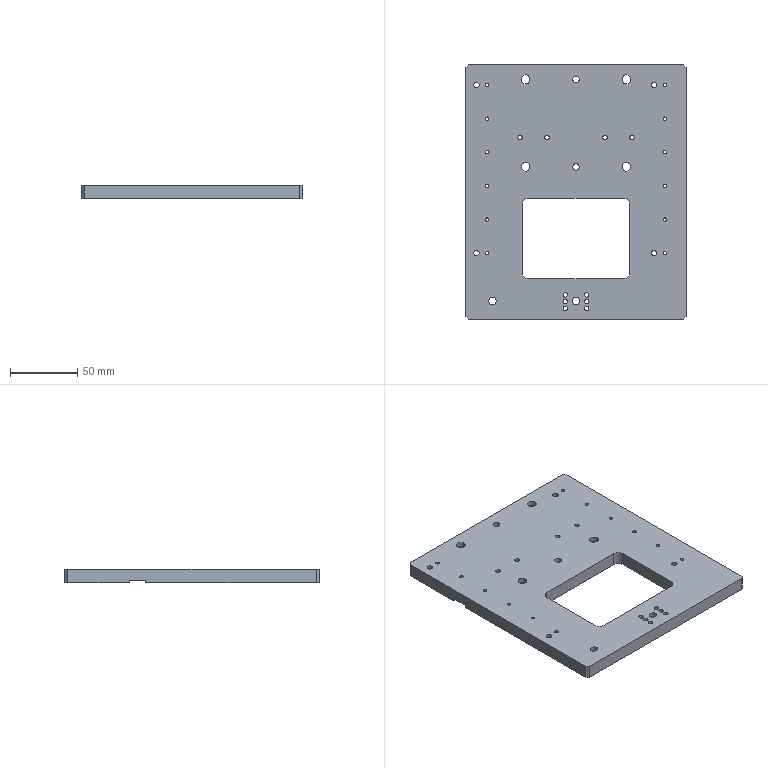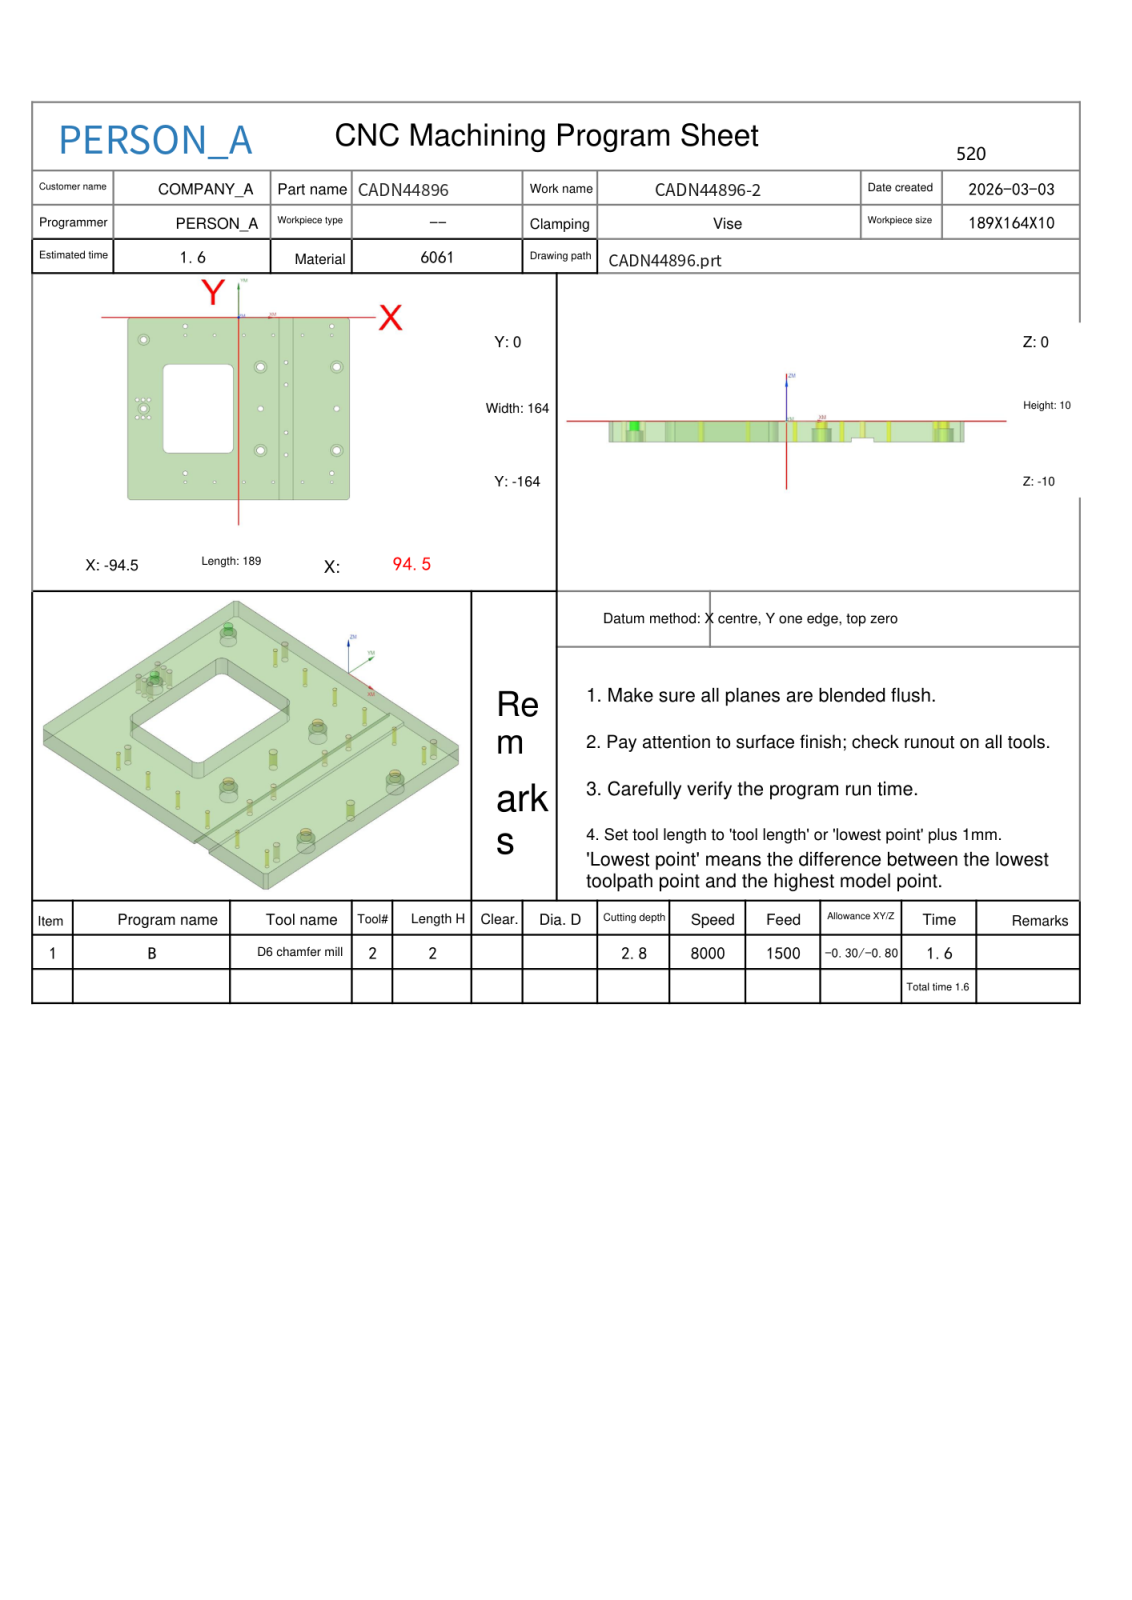NC program | NX | posted by the shop | part box 164 x 189 x 10 mm
Whole program:
%
O0001
(Machine time: 1.67 MIN)
(===Total Tool:1===)
(T2=D6 chamfer mill   D=6.   R=0.   D-  H02 Z=-2.8  )
G80 G90 G17 G49 G40
G91 G28 Z0
M01
N1 T02 M06
(D6 chamfer mill  D=6. R=0. H=02 ce=-0.30 di=0.00)
G00 G90 G54 X-44.338 Y-7.418 M03 S7000
G43 H02 Z50.
M08
Z2.5
G01 X-44.434 Y-7.251 Z2.43 F1500.
X-44.584 Y-7.074 Z2.345
X-44.762 Y-6.926 Z2.261
X-44.964 Y-6.812 Z2.177
X-45.183 Y-6.736 Z2.092
X-45.412 Y-6.7 Z2.008
X-45.588 Z1.944
X-45.817 Y-6.736 Z1.859
X-46.036 Y-6.812 Z1.775
X-46.238 Y-6.926 Z1.691
X-46.416 Y-7.074 Z1.606
X-46.566 Y-7.251 Z1.522
X-46.682 Y-7.451 Z1.438
X-46.76 Y-7.669 Z1.353
X-46.799 Y-7.898 Z1.269
X-46.797 Y-8.13 Z1.185
X-46.753 Y-8.357 Z1.1
X-46.67 Y-8.573 Z1.016
X-46.582 Y-8.727 Z.952
X-46.436 Y-8.907 Z.867
X-46.26 Y-9.058 Z.783
X-46.061 Y-9.176 Z.699
X-45.844 Y-9.257 Z.614
X-45.616 Y-9.298 Z.53
X-45.384 Z.446
X-45.156 Y-9.257 Z.361
X-44.939 Y-9.176 Z.277
X-44.74 Y-9.058 Z.193
X-44.564 Y-8.907 Z.108
X-44.418 Y-8.727 Z.024
X-44.33 Y-8.573 Z-.04
X-44.247 Y-8.357 Z-.125
X-44.203 Y-8.13 Z-.209
X-44.201 Y-7.898 Z-.293
X-44.24 Y-7.669 Z-.378
X-44.318 Y-7.451 Z-.462
X-44.434 Y-7.251 Z-.546
X-44.584 Y-7.074 Z-.631
X-44.762 Y-6.926 Z-.715
X-44.964 Y-6.812 Z-.799
X-45.183 Y-6.736 Z-.884
X-45.412 Y-6.7 Z-.968
X-45.5 Z-1.
G03 X-46.8 Y-8. I0.0 J-1.3
X-45.5 Y-9.3 I1.3 J0.0
X-44.2 Y-8. I0.0 J1.3
X-45.5 Y-6.7 I-1.3 J0.0
X-45.988 Y-6.795 I0.0 J-1.3
G01 Z1.5
G00 Z50.
X-83.051 Y-20.049
Z2.5
G01 X-83.025 Y-20.335 Z2.396
X-82.951 Y-20.639 Z2.281
X-82.831 Y-20.929 Z2.167
X-82.72 Y-21.121 Z2.087
X-82.529 Y-21.37 Z1.973
X-82.303 Y-21.587 Z1.859
X-82.046 Y-21.766 Z1.744
X-81.765 Y-21.905 Z1.63
X-81.466 Y-21.999 Z1.516
X-81.157 Y-22.047 Z1.402
X-80.843 Z1.288
X-80.534 Y-21.999 Z1.174
X-80.235 Y-21.905 Z1.06
X-79.954 Y-21.766 Z.946
X-79.697 Y-21.587 Z.832
X-79.471 Y-21.37 Z.718
X-79.28 Y-21.121 Z.604
X-79.169 Y-20.929 Z.523
X-79.049 Y-20.639 Z.409
X-78.975 Y-20.335 Z.295
X-78.947 Y-20.023 Z.181
X-78.968 Y-19.71 Z.067
X-79.035 Y-19.404 Z-.047
X-79.149 Y-19.112 Z-.161
X-79.306 Y-18.841 Z-.275
X-79.502 Y-18.596 Z-.389
X-79.733 Y-18.385 Z-.503
X-79.993 Y-18.211 Z-.617
X-80.277 Y-18.078 Z-.732
X-80.578 Y-17.991 Z-.846
X-80.889 Y-17.95 Z-.96
X-81. Z-1.
G03 X-83.05 Y-20. I0.0 J-2.05
X-81. Y-22.05 I2.05 J0.0
X-78.95 Y-20. I0.0 J2.05
X-81. Y-17.95 I-2.05 J0.0
X-81.495 Y-18.011 I0.0 J-2.05
G01 Z1.5
G00 Z50.
X-83.051 Y-82.049
Z2.5
G01 X-83.025 Y-82.335 Z2.396
X-82.951 Y-82.639 Z2.281
X-82.831 Y-82.929 Z2.167
X-82.72 Y-83.121 Z2.087
X-82.529 Y-83.37 Z1.973
X-82.303 Y-83.587 Z1.859
X-82.046 Y-83.766 Z1.744
X-81.765 Y-83.905 Z1.63
X-81.466 Y-83.999 Z1.516
X-81.157 Y-84.047 Z1.402
X-80.843 Z1.288
X-80.534 Y-83.999 Z1.174
X-80.235 Y-83.905 Z1.06
X-79.954 Y-83.766 Z.946
X-79.697 Y-83.587 Z.832
X-79.471 Y-83.37 Z.718
X-79.28 Y-83.121 Z.604
X-79.169 Y-82.929 Z.523
X-79.049 Y-82.639 Z.409
X-78.975 Y-82.335 Z.295
X-78.947 Y-82.023 Z.181
X-78.968 Y-81.71 Z.067
X-79.035 Y-81.404 Z-.047
X-79.149 Y-81.112 Z-.161
X-79.306 Y-80.841 Z-.275
X-79.502 Y-80.596 Z-.389
X-79.733 Y-80.385 Z-.503
X-79.993 Y-80.211 Z-.617
X-80.277 Y-80.078 Z-.732
X-80.578 Y-79.991 Z-.846
X-80.889 Y-79.95 Z-.96
X-81. Z-1.
G03 X-83.05 Y-82. I0.0 J-2.05
X-81. Y-84.05 I2.05 J0.0
X-78.95 Y-82. I0.0 J2.05
X-81. Y-79.95 I-2.05 J0.0
X-81.495 Y-80.011 I0.0 J-2.05
G01 Z1.5
G00 Z50.
X-44.338 Y-139.418
Z2.5
G01 X-44.434 Y-139.251 Z2.43
X-44.584 Y-139.074 Z2.345
X-44.762 Y-138.926 Z2.261
X-44.964 Y-138.812 Z2.177
X-45.183 Y-138.736 Z2.092
X-45.412 Y-138.7 Z2.008
X-45.588 Z1.944
X-45.817 Y-138.736 Z1.859
X-46.036 Y-138.812 Z1.775
X-46.238 Y-138.926 Z1.691
X-46.416 Y-139.074 Z1.606
X-46.566 Y-139.251 Z1.522
X-46.682 Y-139.451 Z1.438
X-46.76 Y-139.669 Z1.353
X-46.799 Y-139.898 Z1.269
X-46.797 Y-140.13 Z1.185
X-46.753 Y-140.357 Z1.1
X-46.67 Y-140.573 Z1.016
X-46.582 Y-140.727 Z.952
X-46.436 Y-140.907 Z.867
X-46.26 Y-141.058 Z.783
X-46.061 Y-141.176 Z.699
X-45.844 Y-141.257 Z.614
X-45.616 Y-141.298 Z.53
X-45.384 Z.446
X-45.156 Y-141.257 Z.361
X-44.939 Y-141.176 Z.277
X-44.74 Y-141.058 Z.193
X-44.564 Y-140.907 Z.108
X-44.418 Y-140.727 Z.024
X-44.33 Y-140.573 Z-.04
X-44.247 Y-140.357 Z-.125
X-44.203 Y-140.13 Z-.209
X-44.201 Y-139.898 Z-.293
X-44.24 Y-139.669 Z-.378
X-44.318 Y-139.451 Z-.462
X-44.434 Y-139.251 Z-.546
X-44.584 Y-139.074 Z-.631
X-44.762 Y-138.926 Z-.715
X-44.964 Y-138.812 Z-.799
X-45.183 Y-138.736 Z-.884
X-45.412 Y-138.7 Z-.968
X-45.5 Z-1.
G03 X-46.8 Y-140. I0.0 J-1.3
X-45.5 Y-141.3 I1.3 J0.0
X-44.2 Y-140. I0.0 J1.3
X-45.5 Y-138.7 I-1.3 J0.0
X-45.988 Y-138.795 I0.0 J-1.3
G01 Z1.5
G00 Z50.
X-49.884 Y-42.7
Z2.5
G01 X-59.5 Z-1.
G03 X-63.8 Y-47. I0.0 J-4.3
G01 Y-117.
G03 X-59.5 Y-121.3 I4.3 J0.0
G01 X-9.5
G03 X-5.2 Y-117. I0.0 J4.3
G01 Y-47.
G03 X-9.5 Y-42.7 I-4.3 J0.0
G01 X-59.5
G03 X-59.999 Y-42.729 I0.0 J-4.3
G01 Z1.5
G00 Z50.
X-83.546 Y-164.7
Z2.5
G01 X-92.453 Z-.742
X-92.66 Y-164.662 Z-.819
X-92.855 Y-164.581 Z-.895
X-93.028 Y-164.462 Z-.972
X-93.083 Y-164.407 Z-1.
X-94.907 Y-162.583
G02 X-95.2 Y-161.876 I.707 J.707
G01 Y-2.124
G02 X-94.907 Y-1.417 I1. J0.0
G01 X-93.083 Y.407
G02 X-92.376 Y.7 I.707 J-.707
G01 X92.376
G02 X93.083 Y.407 I0.0 J-1.
G01 X94.907 Y-1.417
G02 X95.2 Y-2.124 I-.707 J-.707
G01 Y-161.876
G02 X94.907 Y-162.583 I-1. J0.0
G01 X93.083 Y-164.407
G02 X92.376 Y-164.7 I-.707 J.707
G01 X-92.376
G02 X-93.083 Y-164.407 I0.0 J1.
G01 X-93.436 Y-164.054
Z1.5
G00 Z50.
X17.33 Y-46.707
Z2.5
G01 X17.53 Y-46.825 Z2.416
X17.849 Y-46.96 Z2.29
X18.183 Y-47.051 Z2.163
X18.527 Y-47.097 Z2.037
X18.873 Z1.911
X19.217 Y-47.051 Z1.785
X19.551 Y-46.96 Z1.659
X19.87 Y-46.825 Z1.533
X20.169 Y-46.649 Z1.407
X20.441 Y-46.435 Z1.281
X20.683 Y-46.187 Z1.154
X20.889 Y-45.908 Z1.028
X21.014 Y-45.692 Z.937
X21.152 Y-45.374 Z.811
X21.246 Y-45.04 Z.685
X21.296 Y-44.697 Z.559
X21.299 Y-44.351 Z.433
X21.256 Y-44.007 Z.307
X21.168 Y-43.672 Z.181
X21.036 Y-43.351 Z.054
X20.863 Y-43.051 Z-.072
X20.651 Y-42.777 Z-.198
X20.405 Y-42.533 Z-.324
X20.128 Y-42.324 Z-.45
X19.827 Y-42.154 Z-.576
X19.505 Y-42.025 Z-.702
X19.169 Y-41.94 Z-.828
X18.825 Y-41.9 Z-.955
X18.7 Z-1.
G03 X16.1 Y-44.5 I0.0 J-2.6
X18.7 Y-47.1 I2.6 J0.0
X21.3 Y-44.5 I0.0 J2.6
X18.7 Y-41.9 I-2.6 J0.0
X18.203 Y-41.948 I0.0 J-2.6
G01 Z1.5
G00 Z50.
X20.159 Y-83.055
Z2.5
G01 X20.188 Y-83.018 Z2.483
X20.325 Y-82.78 Z2.383
X20.425 Y-82.525 Z2.283
X20.485 Y-82.257 Z2.183
X20.503 Y-81.983 Z2.084
X20.48 Y-81.71 Z1.984
X20.415 Y-81.444 Z1.884
X20.311 Y-81.19 Z1.784
X20.207 Y-81.01 Z1.708
X20.039 Y-80.793 Z1.609
X19.841 Y-80.604 Z1.509
X19.616 Y-80.447 Z1.409
X19.37 Y-80.326 Z1.309
X19.108 Y-80.244 Z1.209
X18.837 Y-80.202 Z1.11
X18.563 Z1.01
X18.292 Y-80.244 Z.91
X18.03 Y-80.326 Z.81
X17.784 Y-80.447 Z.71
X17.559 Y-80.604 Z.611
X17.361 Y-80.793 Z.511
X17.193 Y-81.01 Z.411
X17.089 Y-81.19 Z.335
X16.985 Y-81.444 Z.235
X16.92 Y-81.71 Z.136
X16.897 Y-81.983 Z.036
X16.915 Y-82.257 Z-.064
X16.975 Y-82.525 Z-.164
X17.075 Y-82.78 Z-.264
X17.212 Y-83.018 Z-.363
X17.383 Y-83.232 Z-.463
X17.585 Y-83.417 Z-.563
X17.813 Y-83.57 Z-.663
X18.061 Y-83.686 Z-.763
X18.324 Y-83.763 Z-.862
X18.596 Y-83.8 Z-.962
X18.7 Z-1.
G03 X20.5 Y-82. I0.0 J1.8
X18.7 Y-80.2 I-1.8 J0.0
X16.9 Y-82. I0.0 J-1.8
X18.7 Y-83.8 I1.8 J0.0
X19.194 Y-83.731 I0.0 J1.8
G01 Z1.5
G00 Z50.
X17.33 Y-121.707
Z2.5
G01 X17.53 Y-121.825 Z2.416
X17.849 Y-121.96 Z2.29
X18.183 Y-122.051 Z2.163
X18.527 Y-122.097 Z2.037
X18.873 Z1.911
X19.217 Y-122.051 Z1.785
X19.551 Y-121.96 Z1.659
X19.87 Y-121.825 Z1.533
X20.169 Y-121.649 Z1.407
X20.441 Y-121.435 Z1.281
X20.683 Y-121.187 Z1.154
X20.889 Y-120.908 Z1.028
X21.014 Y-120.692 Z.937
X21.152 Y-120.374 Z.811
X21.246 Y-120.04 Z.685
X21.296 Y-119.697 Z.559
X21.299 Y-119.351 Z.433
X21.256 Y-119.007 Z.307
X21.168 Y-118.672 Z.181
X21.036 Y-118.351 Z.054
X20.863 Y-118.051 Z-.072
X20.651 Y-117.777 Z-.198
X20.405 Y-117.533 Z-.324
X20.128 Y-117.324 Z-.45
X19.827 Y-117.154 Z-.576
X19.505 Y-117.025 Z-.702
X19.169 Y-116.94 Z-.828
X18.825 Y-116.9 Z-.955
X18.7 Z-1.
G03 X16.1 Y-119.5 I0.0 J-2.6
X18.7 Y-122.1 I2.6 J0.0
X21.3 Y-119.5 I0.0 J2.6
X18.7 Y-116.9 I-2.6 J0.0
X18.203 Y-116.948 I0.0 J-2.6
G01 Z1.5
G00 Z50.
X80.662 Y-139.418
Z2.5
G01 X80.566 Y-139.251 Z2.43
X80.416 Y-139.074 Z2.345
X80.238 Y-138.926 Z2.261
X80.036 Y-138.812 Z2.177
X79.817 Y-138.736 Z2.092
X79.588 Y-138.7 Z2.008
X79.412 Z1.944
X79.183 Y-138.736 Z1.859
X78.964 Y-138.812 Z1.775
X78.762 Y-138.926 Z1.691
X78.584 Y-139.074 Z1.606
X78.434 Y-139.251 Z1.522
X78.318 Y-139.451 Z1.438
X78.24 Y-139.669 Z1.353
X78.201 Y-139.898 Z1.269
X78.203 Y-140.13 Z1.185
X78.247 Y-140.357 Z1.1
X78.33 Y-140.573 Z1.016
X78.418 Y-140.727 Z.952
X78.564 Y-140.907 Z.867
X78.74 Y-141.058 Z.783
X78.939 Y-141.176 Z.699
X79.156 Y-141.257 Z.614
X79.384 Y-141.298 Z.53
X79.616 Z.446
X79.844 Y-141.257 Z.361
X80.061 Y-141.176 Z.277
X80.26 Y-141.058 Z.193
X80.436 Y-140.907 Z.108
X80.582 Y-140.727 Z.024
X80.67 Y-140.573 Z-.04
X80.753 Y-140.357 Z-.125
X80.797 Y-140.13 Z-.209
X80.799 Y-139.898 Z-.293
X80.76 Y-139.669 Z-.378
X80.682 Y-139.451 Z-.462
X80.566 Y-139.251 Z-.546
X80.416 Y-139.074 Z-.631
X80.238 Y-138.926 Z-.715
X80.036 Y-138.812 Z-.799
X79.817 Y-138.736 Z-.884
X79.588 Y-138.7 Z-.968
X79.5 Z-1.
G03 X78.2 Y-140. I0.0 J-1.3
X79.5 Y-141.3 I1.3 J0.0
X80.8 Y-140. I0.0 J1.3
X79.5 Y-138.7 I-1.3 J0.0
X79.012 Y-138.795 I0.0 J-1.3
G01 Z1.5
G00 Z50.
X82.33 Y-121.707
Z2.5
G01 X82.53 Y-121.825 Z2.416
X82.849 Y-121.96 Z2.29
X83.183 Y-122.051 Z2.163
X83.527 Y-122.097 Z2.037
X83.873 Z1.911
X84.217 Y-122.051 Z1.785
X84.551 Y-121.96 Z1.659
X84.87 Y-121.825 Z1.533
X85.169 Y-121.649 Z1.407
X85.441 Y-121.435 Z1.281
X85.683 Y-121.187 Z1.154
X85.889 Y-120.908 Z1.028
X86.014 Y-120.692 Z.937
X86.152 Y-120.374 Z.811
X86.246 Y-120.04 Z.685
X86.296 Y-119.697 Z.559
X86.299 Y-119.351 Z.433
X86.256 Y-119.007 Z.307
X86.168 Y-118.672 Z.181
X86.036 Y-118.351 Z.054
X85.863 Y-118.051 Z-.072
X85.651 Y-117.777 Z-.198
X85.405 Y-117.533 Z-.324
X85.128 Y-117.324 Z-.45
X84.827 Y-117.154 Z-.576
X84.505 Y-117.025 Z-.702
X84.169 Y-116.94 Z-.828
X83.825 Y-116.9 Z-.955
X83.7 Z-1.
G03 X81.1 Y-119.5 I0.0 J-2.6
X83.7 Y-122.1 I2.6 J0.0
X86.3 Y-119.5 I0.0 J2.6
X83.7 Y-116.9 I-2.6 J0.0
X83.203 Y-116.948 I0.0 J-2.6
G01 Z1.5
G00 Z50.
X85.159 Y-83.055
Z2.5
G01 X85.188 Y-83.018 Z2.483
X85.325 Y-82.78 Z2.383
X85.425 Y-82.525 Z2.283
X85.485 Y-82.257 Z2.183
X85.503 Y-81.983 Z2.084
X85.48 Y-81.71 Z1.984
X85.415 Y-81.444 Z1.884
X85.311 Y-81.19 Z1.784
X85.207 Y-81.01 Z1.708
X85.039 Y-80.793 Z1.609
X84.841 Y-80.604 Z1.509
X84.616 Y-80.447 Z1.409
X84.37 Y-80.326 Z1.309
X84.108 Y-80.244 Z1.209
X83.837 Y-80.202 Z1.11
X83.563 Z1.01
X83.292 Y-80.244 Z.91
X83.03 Y-80.326 Z.81
X82.784 Y-80.447 Z.71
X82.559 Y-80.604 Z.611
X82.361 Y-80.793 Z.511
X82.193 Y-81.01 Z.411
X82.089 Y-81.19 Z.335
X81.985 Y-81.444 Z.235
X81.92 Y-81.71 Z.136
X81.897 Y-81.983 Z.036
X81.915 Y-82.257 Z-.064
X81.975 Y-82.525 Z-.164
X82.075 Y-82.78 Z-.264
X82.212 Y-83.018 Z-.363
X82.383 Y-83.232 Z-.463
X82.585 Y-83.417 Z-.563
X82.813 Y-83.57 Z-.663
X83.061 Y-83.686 Z-.763
X83.324 Y-83.763 Z-.862
X83.596 Y-83.8 Z-.962
X83.7 Z-1.
G03 X85.5 Y-82. I0.0 J1.8
X83.7 Y-80.2 I-1.8 J0.0
X81.9 Y-82. I0.0 J-1.8
X83.7 Y-83.8 I1.8 J0.0
X84.194 Y-83.731 I0.0 J1.8
G01 Z1.5
G00 Z50.
X82.33 Y-46.707
Z2.5
G01 X82.53 Y-46.825 Z2.416
X82.849 Y-46.96 Z2.29
X83.183 Y-47.051 Z2.163
X83.527 Y-47.097 Z2.037
X83.873 Z1.911
X84.217 Y-47.051 Z1.785
X84.551 Y-46.96 Z1.659
X84.87 Y-46.825 Z1.533
X85.169 Y-46.649 Z1.407
X85.441 Y-46.435 Z1.281
X85.683 Y-46.187 Z1.154
X85.889 Y-45.908 Z1.028
X86.014 Y-45.692 Z.937
X86.152 Y-45.374 Z.811
X86.246 Y-45.04 Z.685
X86.296 Y-44.697 Z.559
X86.299 Y-44.351 Z.433
X86.256 Y-44.007 Z.307
X86.168 Y-43.672 Z.181
X86.036 Y-43.351 Z.054
X85.863 Y-43.051 Z-.072
X85.651 Y-42.777 Z-.198
X85.405 Y-42.533 Z-.324
X85.128 Y-42.324 Z-.45
X84.827 Y-42.154 Z-.576
X84.505 Y-42.025 Z-.702
X84.169 Y-41.94 Z-.828
X83.825 Y-41.9 Z-.955
X83.7 Z-1.
G03 X81.1 Y-44.5 I0.0 J-2.6
X83.7 Y-47.1 I2.6 J0.0
X86.3 Y-44.5 I0.0 J2.6
X83.7 Y-41.9 I-2.6 J0.0
X83.203 Y-41.948 I0.0 J-2.6
G01 Z1.5
G00 Z50.
X80.662 Y-7.418
Z2.5
G01 X80.566 Y-7.251 Z2.43
X80.416 Y-7.074 Z2.345
X80.238 Y-6.926 Z2.261
X80.036 Y-6.812 Z2.177
X79.817 Y-6.736 Z2.092
X79.588 Y-6.7 Z2.008
X79.412 Z1.944
X79.183 Y-6.736 Z1.859
X78.964 Y-6.812 Z1.775
X78.762 Y-6.926 Z1.691
X78.584 Y-7.074 Z1.606
X78.434 Y-7.251 Z1.522
X78.318 Y-7.451 Z1.438
X78.24 Y-7.669 Z1.353
X78.201 Y-7.898 Z1.269
X78.203 Y-8.13 Z1.185
X78.247 Y-8.357 Z1.1
X78.33 Y-8.573 Z1.016
X78.418 Y-8.727 Z.952
X78.564 Y-8.907 Z.867
X78.74 Y-9.058 Z.783
X78.939 Y-9.176 Z.699
X79.156 Y-9.257 Z.614
X79.384 Y-9.298 Z.53
X79.616 Z.446
X79.844 Y-9.257 Z.361
X80.061 Y-9.176 Z.277
X80.26 Y-9.058 Z.193
X80.436 Y-8.907 Z.108
X80.582 Y-8.727 Z.024
X80.67 Y-8.573 Z-.04
X80.753 Y-8.357 Z-.125
X80.797 Y-8.13 Z-.209
X80.799 Y-7.898 Z-.293
X80.76 Y-7.669 Z-.378
X80.682 Y-7.451 Z-.462
X80.566 Y-7.251 Z-.546
X80.416 Y-7.074 Z-.631
X80.238 Y-6.926 Z-.715
X80.036 Y-6.812 Z-.799
X79.817 Y-6.736 Z-.884
X79.588 Y-6.7 Z-.968
X79.5 Z-1.
G03 X78.2 Y-8. I0.0 J-1.3
X79.5 Y-9.3 I1.3 J0.0
X80.8 Y-8. I0.0 J1.3
X79.5 Y-6.7 I-1.3 J0.0
X79.012 Y-6.795 I0.0 J-1.3
G01 Z1.5
G00 Z50.
G00 G90 X79.5 Y-148. M03 S8000
Z50.
G98 G81 X79.5 Y-148. Z-1.75 R3. F1000.
X54.5
X29.5
X4.5
X-20.5
X-45.5
Y-16.
X-20.5
X4.5
X29.5
X54.5
X79.5
G80
G00 Z50.
G00 G90 X40.5 Y-40.5 M03 S8000
Z50.
G98 G81 X40.5 Y-40.5 Z-2.2 R3. F1000.
Y-60.5
Y-103.5
Y-123.5
X-76.5 Y-90.
X-81.5
X-86.5
Y-74.
X-81.5
X-76.5
G80
G00 Z50.
G00 G90 X79.5 Y-8. M03 S8000
Z50.
G98 G81 X79.5 Y-8. Z-2.3 R3. F1000.
X-45.5
Y-140.
X79.5
G80
G00 Z50.
G00 G90 X18.7 Y-82. M03 S8000
Z50.
G98 G81 X18.7 Y-82. Z-2.8 R3. F1000.
X83.7
G80
G00 Z50.
G00 G90 X-81.647 Y-20.065 M03 S8000
Z50.
Z-.9
G01 Z-1.4 F1200.
X-82.5 Y-20.15
G03 X-81. Y-21.65 I1.5 J0.0
X-79.35 Y-20. I0.0 J1.65
X-81. Y-18.35 I-1.65 J0.0
X-82.65 Y-20. I0.0 J-1.65
X-81. Y-21.65 I1.65 J0.0
X-79.5 Y-20.15 I0.0 J1.5
G01 X-80.353 Y-20.065
Z-.9
G00 Z50.
X-81.647 Y-82.065
Z-.9
G01 Z-1.4
X-82.5 Y-82.15
G03 X-81. Y-83.65 I1.5 J0.0
X-79.35 Y-82. I0.0 J1.65
X-81. Y-80.35 I-1.65 J0.0
X-82.65 Y-82. I0.0 J-1.65
X-81. Y-83.65 I1.65 J0.0
X-79.5 Y-82.15 I0.0 J1.5
G01 X-80.353 Y-82.065
Z-.9
G00 Z50.
G00 G90 X17.613 Y-120.007 M03 S8000
Z50.
Z-.9
G01 Z-1.4 F1200.
X17.2 Y-120.2
G03 X18.7 Y-121.7 I1.5 J0.0
X20.9 Y-119.5 I0.0 J2.2
X18.7 Y-117.3 I-2.2 J0.0
X16.5 Y-119.5 I0.0 J-2.2
X18.7 Y-121.7 I2.2 J0.0
X20.2 Y-120.2 I0.0 J1.5
G01 X19.787 Y-120.007
Z-.9
G00 Z50.
X82.613
Z-.9
G01 Z-1.4
X82.2 Y-120.2
G03 X83.7 Y-121.7 I1.5 J0.0
X85.9 Y-119.5 I0.0 J2.2
X83.7 Y-117.3 I-2.2 J0.0
X81.5 Y-119.5 I0.0 J-2.2
X83.7 Y-121.7 I2.2 J0.0
X85.2 Y-120.2 I0.0 J1.5
G01 X84.787 Y-120.007
Z-.9
G00 Z50.
X82.613 Y-45.007
Z-.9
G01 Z-1.4
X82.2 Y-45.2
G03 X83.7 Y-46.7 I1.5 J0.0
X85.9 Y-44.5 I0.0 J2.2
X83.7 Y-42.3 I-2.2 J0.0
X81.5 Y-44.5 I0.0 J-2.2
X83.7 Y-46.7 I2.2 J0.0
X85.2 Y-45.2 I0.0 J1.5
G01 X84.787 Y-45.007
Z-.9
G00 Z50.
X17.613
Z-.9
G01 Z-1.4
X17.2 Y-45.2
G03 X18.7 Y-46.7 I1.5 J0.0
X20.9 Y-44.5 I0.0 J2.2
X18.7 Y-42.3 I-2.2 J0.0
X16.5 Y-44.5 I0.0 J-2.2
X18.7 Y-46.7 I2.2 J0.0
X20.2 Y-45.2 I0.0 J1.5
G01 X19.787 Y-45.007
Z-.9
G00 Z50.
M05
M09
G91 G28 Z0.0
G91 G28 Y0.0
M30
%